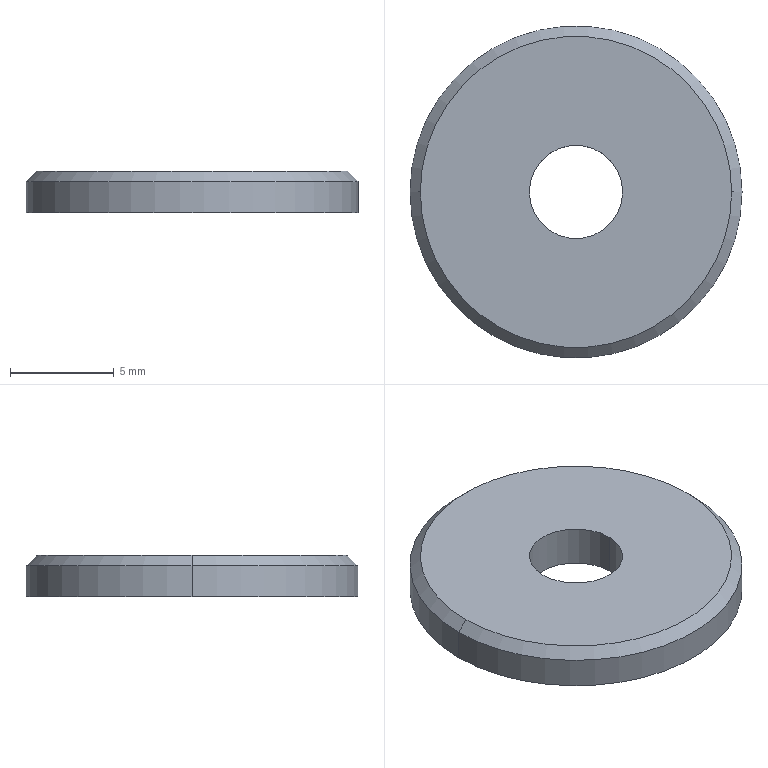Part | STEP file | Gland cover^Driven wheel assembly | 1 solid | 8 faces | box 16 x 16 x 2 mm | volume 364.163 mm3 | cylinder 4 | cone 2 | plane 2 | commonest cylinder face diameters 4.5 x2 16 x2
STEP:
#1=CARTESIAN_POINT('',(-2.25,0.,18.3));
#2=VERTEX_POINT('',#1);
#3=CARTESIAN_POINT('',(2.25,0.,18.3));
#4=VERTEX_POINT('',#3);
#5=CARTESIAN_POINT('',(0.,0.,18.3));
#6=DIRECTION('',(0.,0.,1.));
#7=DIRECTION('',(1.,0.,0.));
#8=AXIS2_PLACEMENT_3D('',#5,#6,#7);
#9=CIRCLE('',#8,2.25);
#10=EDGE_CURVE('',#2,#4,#9,.T.);
#11=ORIENTED_EDGE('',*,*,#10,.F.);
#12=CARTESIAN_POINT('',(-2.25,0.,20.3));
#13=VERTEX_POINT('',#12);
#14=CARTESIAN_POINT('',(-2.25,0.,20.3));
#15=DIRECTION('',(0.,0.,1.));
#16=VECTOR('',#15,1000.);
#17=LINE('',#14,#16);
#18=EDGE_CURVE('',#2,#13,#17,.T.);
#19=ORIENTED_EDGE('',*,*,#18,.T.);
#20=CARTESIAN_POINT('',(2.25,0.,20.3));
#21=VERTEX_POINT('',#20);
#22=CARTESIAN_POINT('',(0.,0.,20.3));
#23=DIRECTION('',(0.,0.,1.));
#24=DIRECTION('',(1.,0.,0.));
#25=AXIS2_PLACEMENT_3D('',#22,#23,#24);
#26=CIRCLE('',#25,2.25);
#27=EDGE_CURVE('',#13,#21,#26,.T.);
#28=ORIENTED_EDGE('',*,*,#27,.T.);
#29=CARTESIAN_POINT('',(2.25,0.,20.3));
#30=DIRECTION('',(0.,0.,1.));
#31=VECTOR('',#30,1000.);
#32=LINE('',#29,#31);
#33=EDGE_CURVE('',#4,#21,#32,.T.);
#34=ORIENTED_EDGE('',*,*,#33,.F.);
#35=EDGE_LOOP('',(#11,#19,#28,#34));
#36=FACE_OUTER_BOUND('',#35,.T.);
#37=CARTESIAN_POINT('',(0.,0.,20.3));
#38=DIRECTION('',(0.,0.,1.));
#39=DIRECTION('',(1.,0.,0.));
#40=AXIS2_PLACEMENT_3D('',#37,#38,#39);
#41=CYLINDRICAL_SURFACE('',#40,2.25);
#42=ADVANCED_FACE('',(#36),#41,.F.);
#43=CARTESIAN_POINT('',(7.5,0.,20.3));
#44=VERTEX_POINT('',#43);
#45=CARTESIAN_POINT('',(-7.5,0.,20.3));
#46=VERTEX_POINT('',#45);
#47=CARTESIAN_POINT('',(0.,0.,20.3));
#48=DIRECTION('',(0.,0.,1.));
#49=DIRECTION('',(1.,0.,0.));
#50=AXIS2_PLACEMENT_3D('',#47,#48,#49);
#51=CIRCLE('',#50,7.5);
#52=EDGE_CURVE('',#44,#46,#51,.T.);
#53=ORIENTED_EDGE('',*,*,#52,.F.);
#54=CARTESIAN_POINT('',(8.,0.,19.8));
#55=VERTEX_POINT('',#54);
#56=CARTESIAN_POINT('',(7.5,0.,20.3));
#57=DIRECTION('',(0.7071,0.,-0.7071));
#58=VECTOR('',#57,1000.);
#59=LINE('',#56,#58);
#60=EDGE_CURVE('',#44,#55,#59,.T.);
#61=ORIENTED_EDGE('',*,*,#60,.T.);
#62=CARTESIAN_POINT('',(-8.,0.,19.8));
#63=VERTEX_POINT('',#62);
#64=CARTESIAN_POINT('',(0.,0.,19.8));
#65=DIRECTION('',(0.,0.,-1.));
#66=DIRECTION('',(1.,0.,0.));
#67=AXIS2_PLACEMENT_3D('',#64,#65,#66);
#68=CIRCLE('',#67,8.);
#69=EDGE_CURVE('',#63,#55,#68,.T.);
#70=ORIENTED_EDGE('',*,*,#69,.F.);
#71=CARTESIAN_POINT('',(-7.5,0.,20.3));
#72=DIRECTION('',(-0.7071,0.,-0.7071));
#73=VECTOR('',#72,1000.);
#74=LINE('',#71,#73);
#75=EDGE_CURVE('',#46,#63,#74,.T.);
#76=ORIENTED_EDGE('',*,*,#75,.F.);
#77=EDGE_LOOP('',(#53,#61,#70,#76));
#78=FACE_OUTER_BOUND('',#77,.T.);
#79=CARTESIAN_POINT('',(0.,0.,20.3));
#80=DIRECTION('',(0.,0.,-1.));
#81=DIRECTION('',(-1.,0.,0.));
#82=AXIS2_PLACEMENT_3D('',#79,#80,#81);
#83=CONICAL_SURFACE('',#82,7.5,0.7854);
#84=ADVANCED_FACE('',(#78),#83,.T.);
#85=ORIENTED_EDGE('',*,*,#69,.T.);
#86=CARTESIAN_POINT('',(8.,0.,18.3));
#87=VERTEX_POINT('',#86);
#88=CARTESIAN_POINT('',(8.,0.,20.3));
#89=DIRECTION('',(0.,0.,-1.));
#90=VECTOR('',#89,1000.);
#91=LINE('',#88,#90);
#92=EDGE_CURVE('',#55,#87,#91,.T.);
#93=ORIENTED_EDGE('',*,*,#92,.T.);
#94=CARTESIAN_POINT('',(-8.,0.,18.3));
#95=VERTEX_POINT('',#94);
#96=CARTESIAN_POINT('',(0.,0.,18.3));
#97=DIRECTION('',(0.,0.,1.));
#98=DIRECTION('',(1.,0.,0.));
#99=AXIS2_PLACEMENT_3D('',#96,#97,#98);
#100=CIRCLE('',#99,8.);
#101=EDGE_CURVE('',#87,#95,#100,.T.);
#102=ORIENTED_EDGE('',*,*,#101,.T.);
#103=CARTESIAN_POINT('',(-8.,0.,20.3));
#104=DIRECTION('',(0.,0.,-1.));
#105=VECTOR('',#104,1000.);
#106=LINE('',#103,#105);
#107=EDGE_CURVE('',#63,#95,#106,.T.);
#108=ORIENTED_EDGE('',*,*,#107,.F.);
#109=EDGE_LOOP('',(#85,#93,#102,#108));
#110=FACE_OUTER_BOUND('',#109,.T.);
#111=CARTESIAN_POINT('',(0.,0.,20.3));
#112=DIRECTION('',(0.,0.,-1.));
#113=DIRECTION('',(-1.,0.,0.));
#114=AXIS2_PLACEMENT_3D('',#111,#112,#113);
#115=CYLINDRICAL_SURFACE('',#114,8.);
#116=ADVANCED_FACE('',(#110),#115,.T.);
#117=ORIENTED_EDGE('',*,*,#92,.F.);
#118=CARTESIAN_POINT('',(0.,0.,19.8));
#119=DIRECTION('',(0.,0.,-1.));
#120=DIRECTION('',(1.,0.,0.));
#121=AXIS2_PLACEMENT_3D('',#118,#119,#120);
#122=CIRCLE('',#121,8.);
#123=EDGE_CURVE('',#55,#63,#122,.T.);
#124=ORIENTED_EDGE('',*,*,#123,.T.);
#125=ORIENTED_EDGE('',*,*,#107,.T.);
#126=CARTESIAN_POINT('',(0.,0.,18.3));
#127=DIRECTION('',(0.,0.,1.));
#128=DIRECTION('',(1.,0.,0.));
#129=AXIS2_PLACEMENT_3D('',#126,#127,#128);
#130=CIRCLE('',#129,8.);
#131=EDGE_CURVE('',#95,#87,#130,.T.);
#132=ORIENTED_EDGE('',*,*,#131,.T.);
#133=EDGE_LOOP('',(#117,#124,#125,#132));
#134=FACE_OUTER_BOUND('',#133,.T.);
#135=CARTESIAN_POINT('',(0.,0.,20.3));
#136=DIRECTION('',(0.,0.,-1.));
#137=DIRECTION('',(-1.,0.,0.));
#138=AXIS2_PLACEMENT_3D('',#135,#136,#137);
#139=CYLINDRICAL_SURFACE('',#138,8.);
#140=ADVANCED_FACE('',(#134),#139,.T.);
#141=CARTESIAN_POINT('',(0.,0.,20.3));
#142=DIRECTION('',(0.,0.,1.));
#143=DIRECTION('',(1.,0.,0.));
#144=AXIS2_PLACEMENT_3D('',#141,#142,#143);
#145=CIRCLE('',#144,2.25);
#146=EDGE_CURVE('',#21,#13,#145,.T.);
#147=ORIENTED_EDGE('',*,*,#146,.F.);
#148=ORIENTED_EDGE('',*,*,#27,.F.);
#149=EDGE_LOOP('',(#147,#148));
#150=FACE_BOUND('',#149,.T.);
#151=CARTESIAN_POINT('',(0.,0.,20.3));
#152=DIRECTION('',(0.,0.,1.));
#153=DIRECTION('',(1.,0.,0.));
#154=AXIS2_PLACEMENT_3D('',#151,#152,#153);
#155=CIRCLE('',#154,7.5);
#156=EDGE_CURVE('',#46,#44,#155,.T.);
#157=ORIENTED_EDGE('',*,*,#156,.T.);
#158=ORIENTED_EDGE('',*,*,#52,.T.);
#159=EDGE_LOOP('',(#157,#158));
#160=FACE_OUTER_BOUND('',#159,.T.);
#161=CARTESIAN_POINT('',(0.,0.,20.3));
#162=DIRECTION('',(0.,0.,1.));
#163=DIRECTION('',(1.,0.,0.));
#164=AXIS2_PLACEMENT_3D('',#161,#162,#163);
#165=PLANE('',#164);
#166=ADVANCED_FACE('',(#150,#160),#165,.T.);
#167=CARTESIAN_POINT('',(0.,0.,18.3));
#168=DIRECTION('',(0.,0.,1.));
#169=DIRECTION('',(1.,0.,0.));
#170=AXIS2_PLACEMENT_3D('',#167,#168,#169);
#171=CIRCLE('',#170,2.25);
#172=EDGE_CURVE('',#4,#2,#171,.T.);
#173=ORIENTED_EDGE('',*,*,#172,.T.);
#174=ORIENTED_EDGE('',*,*,#10,.T.);
#175=EDGE_LOOP('',(#173,#174));
#176=FACE_BOUND('',#175,.T.);
#177=ORIENTED_EDGE('',*,*,#131,.F.);
#178=ORIENTED_EDGE('',*,*,#101,.F.);
#179=EDGE_LOOP('',(#177,#178));
#180=FACE_OUTER_BOUND('',#179,.T.);
#181=CARTESIAN_POINT('',(0.,0.,18.3));
#182=DIRECTION('',(0.,0.,1.));
#183=DIRECTION('',(1.,0.,0.));
#184=AXIS2_PLACEMENT_3D('',#181,#182,#183);
#185=PLANE('',#184);
#186=ADVANCED_FACE('',(#176,#180),#185,.F.);
#187=ORIENTED_EDGE('',*,*,#60,.F.);
#188=ORIENTED_EDGE('',*,*,#156,.F.);
#189=ORIENTED_EDGE('',*,*,#75,.T.);
#190=ORIENTED_EDGE('',*,*,#123,.F.);
#191=EDGE_LOOP('',(#187,#188,#189,#190));
#192=FACE_OUTER_BOUND('',#191,.T.);
#193=CARTESIAN_POINT('',(0.,0.,20.3));
#194=DIRECTION('',(0.,0.,-1.));
#195=DIRECTION('',(-1.,0.,0.));
#196=AXIS2_PLACEMENT_3D('',#193,#194,#195);
#197=CONICAL_SURFACE('',#196,7.5,0.7854);
#198=ADVANCED_FACE('',(#192),#197,.T.);
#199=ORIENTED_EDGE('',*,*,#18,.F.);
#200=ORIENTED_EDGE('',*,*,#172,.F.);
#201=ORIENTED_EDGE('',*,*,#33,.T.);
#202=ORIENTED_EDGE('',*,*,#146,.T.);
#203=EDGE_LOOP('',(#199,#200,#201,#202));
#204=FACE_OUTER_BOUND('',#203,.T.);
#205=CARTESIAN_POINT('',(0.,0.,20.3));
#206=DIRECTION('',(0.,0.,1.));
#207=DIRECTION('',(1.,0.,0.));
#208=AXIS2_PLACEMENT_3D('',#205,#206,#207);
#209=CYLINDRICAL_SURFACE('',#208,2.25);
#210=ADVANCED_FACE('',(#204),#209,.F.);
#211=CLOSED_SHELL('',(#42,#84,#116,#140,#166,#186,#198,#210));
#212=MANIFOLD_SOLID_BREP('',#211);
#213=CARTESIAN_POINT('',(0.,0.,0.));
#214=DIRECTION('',(0.,0.,1.));
#215=DIRECTION('',(1.,0.,0.));
#216=AXIS2_PLACEMENT_3D('',#213,#214,#215);
#217=(LENGTH_UNIT()NAMED_UNIT(*)SI_UNIT(.MILLI.,.METRE.));
#218=UNCERTAINTY_MEASURE_WITH_UNIT(LENGTH_MEASURE(0.00001),#217,'','');
#219=(NAMED_UNIT(*)PLANE_ANGLE_UNIT()SI_UNIT($,.RADIAN.));
#220=(NAMED_UNIT(*)SI_UNIT($,.STERADIAN.)SOLID_ANGLE_UNIT());
#221=(GEOMETRIC_REPRESENTATION_CONTEXT(3)GLOBAL_UNCERTAINTY_ASSIGNED_CONTEXT((#218))GLOBAL_UNIT_ASSIGNED_CONTEXT((#217,#219,#220))REPRESENTATION_CONTEXT('',''));
#222=ADVANCED_BREP_SHAPE_REPRESENTATION('',(#212,#216),#221);